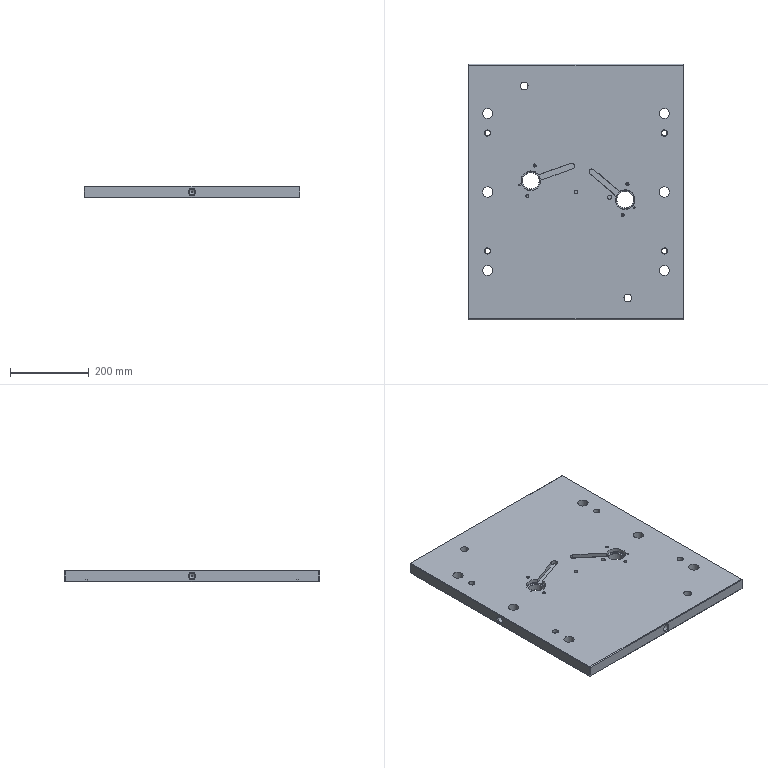Part | STEP file | P011002A002-000 | 1 solid | 502 faces | box 550 x 650 x 30 mm | volume 10420877 mm3 | plane 340 | cylinder 62 | other 53 | cone 47 | commonest cylinder face diameters 16 x8 26 x6 5 x4 6.8 x4 7.973 x4 8 x4